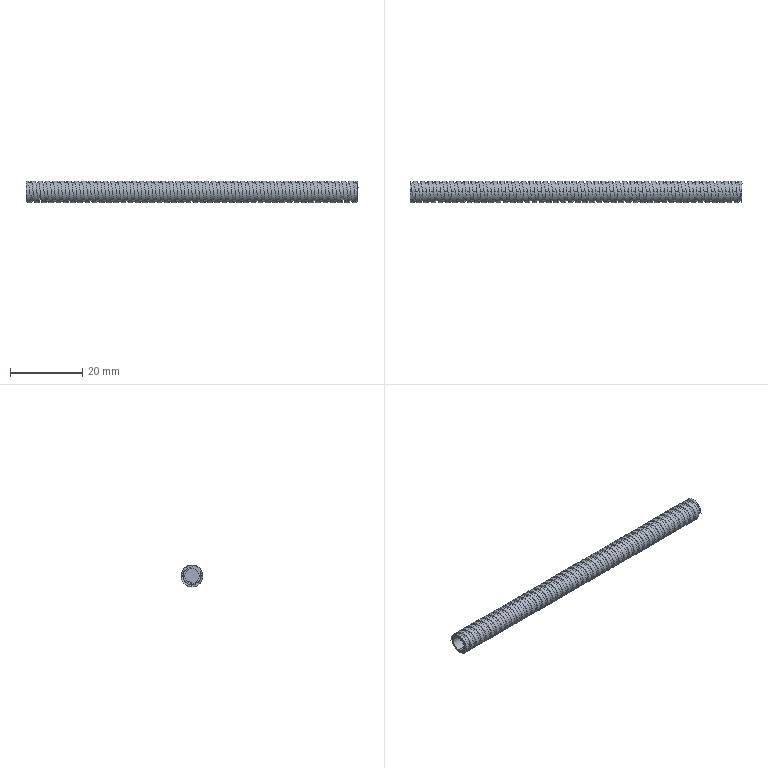Part | SolidWorks | features ICE 2, Cut 1, Helix 1, Revolution 1, SweepCut 1 | 1 solid | 102 faces | box 92 x 6 x 6 mm | volume 2029 mm3 | cylinder 96 | plane 3 | spline 3 | commonest cylinder face diameters 6 x94 4 x2